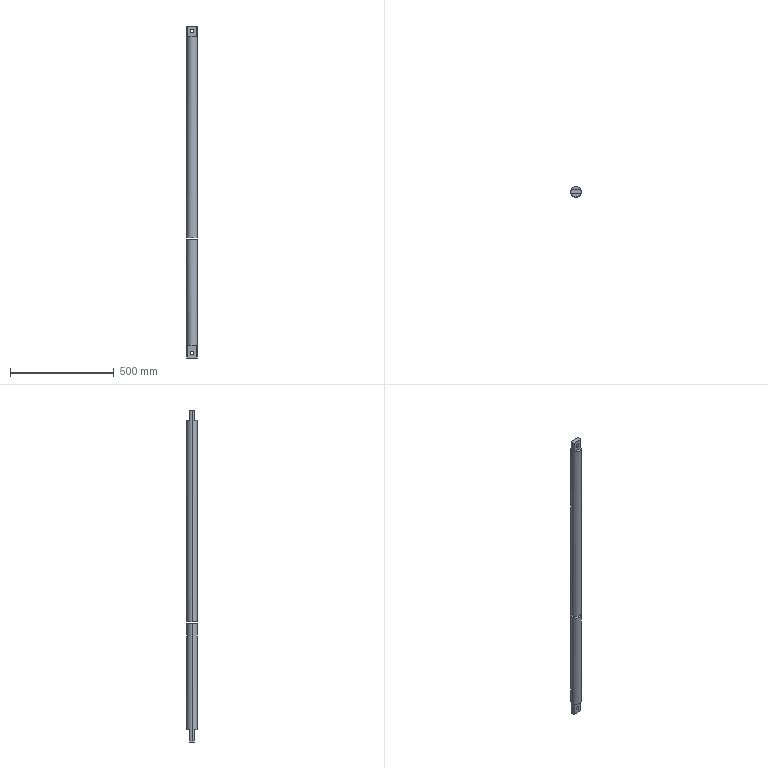Part | SolidWorks | features HoleWzd 2, ICE 2, MirrorPattern 2, Extrusion 1 | 2 solids | 20 faces | box 50 x 50 x 1600 mm | volume 3004412 mm3 | plane 12 | cylinder 8 | commonest cylinder face diameters 16.5 x4 50 x4
STEP:
#1=CARTESIAN_POINT('',(0.,10.,33.25));
#2=VERTEX_POINT('',#1);
#3=CARTESIAN_POINT('',(0.,10.,16.75));
#4=VERTEX_POINT('',#3);
#5=CARTESIAN_POINT('',(0.,10.,25.));
#6=DIRECTION('',(0.,-1.,0.));
#7=DIRECTION('',(0.,0.,-1.));
#8=AXIS2_PLACEMENT_3D('',#5,#6,#7);
#9=CIRCLE('',#8,8.25);
#10=EDGE_CURVE('',#2,#4,#9,.T.);
#11=ORIENTED_EDGE('',*,*,#10,.F.);
#12=CARTESIAN_POINT('',(0.,-10.,33.25));
#13=VERTEX_POINT('',#12);
#14=CARTESIAN_POINT('',(0.,-10.,33.25));
#15=DIRECTION('',(0.,-1.,0.));
#16=VECTOR('',#15,1000.);
#17=LINE('',#14,#16);
#18=EDGE_CURVE('',#2,#13,#17,.T.);
#19=ORIENTED_EDGE('',*,*,#18,.T.);
#20=CARTESIAN_POINT('',(0.,-10.,16.75));
#21=VERTEX_POINT('',#20);
#22=CARTESIAN_POINT('',(0.,-10.,25.));
#23=DIRECTION('',(0.,-1.,0.));
#24=DIRECTION('',(0.,0.,-1.));
#25=AXIS2_PLACEMENT_3D('',#22,#23,#24);
#26=CIRCLE('',#25,8.25);
#27=EDGE_CURVE('',#13,#21,#26,.T.);
#28=ORIENTED_EDGE('',*,*,#27,.T.);
#29=CARTESIAN_POINT('',(0.,-10.,16.75));
#30=DIRECTION('',(0.,-1.,0.));
#31=VECTOR('',#30,1000.);
#32=LINE('',#29,#31);
#33=EDGE_CURVE('',#4,#21,#32,.T.);
#34=ORIENTED_EDGE('',*,*,#33,.F.);
#35=EDGE_LOOP('',(#11,#19,#28,#34));
#36=FACE_OUTER_BOUND('',#35,.T.);
#37=CARTESIAN_POINT('',(0.,-10.,25.));
#38=DIRECTION('',(0.,-1.,0.));
#39=DIRECTION('',(0.,0.,-1.));
#40=AXIS2_PLACEMENT_3D('',#37,#38,#39);
#41=CYLINDRICAL_SURFACE('',#40,8.25);
#42=ADVANCED_FACE('',(#36),#41,.F.);
#43=CARTESIAN_POINT('',(25.,0.,569.));
#44=VERTEX_POINT('',#43);
#45=CARTESIAN_POINT('',(-25.,0.,569.));
#46=VERTEX_POINT('',#45);
#47=CARTESIAN_POINT('',(0.,0.,569.));
#48=DIRECTION('',(0.,0.,1.));
#49=DIRECTION('',(0.,-1.,0.));
#50=AXIS2_PLACEMENT_3D('',#47,#48,#49);
#51=CIRCLE('',#50,25.);
#52=EDGE_CURVE('',#44,#46,#51,.T.);
#53=ORIENTED_EDGE('',*,*,#52,.F.);
#54=CARTESIAN_POINT('',(25.,0.,0.));
#55=VERTEX_POINT('',#54);
#56=CARTESIAN_POINT('',(25.,0.,1600.));
#57=DIRECTION('',(0.,0.,-1.));
#58=VECTOR('',#57,1000.);
#59=LINE('',#56,#58);
#60=EDGE_CURVE('',#44,#55,#59,.T.);
#61=ORIENTED_EDGE('',*,*,#60,.T.);
#62=CARTESIAN_POINT('',(22.913,10.,0.));
#63=VERTEX_POINT('',#62);
#64=CARTESIAN_POINT('',(0.,0.,0.));
#65=DIRECTION('',(0.,0.,1.));
#66=DIRECTION('',(1.,0.,0.));
#67=AXIS2_PLACEMENT_3D('',#64,#65,#66);
#68=CIRCLE('',#67,25.);
#69=EDGE_CURVE('',#55,#63,#68,.T.);
#70=ORIENTED_EDGE('',*,*,#69,.T.);
#71=CARTESIAN_POINT('',(22.913,10.,60.));
#72=VERTEX_POINT('',#71);
#73=CARTESIAN_POINT('',(22.913,10.,1600.));
#74=DIRECTION('',(0.,0.,1.));
#75=VECTOR('',#74,1000.);
#76=LINE('',#73,#75);
#77=EDGE_CURVE('',#63,#72,#76,.T.);
#78=ORIENTED_EDGE('',*,*,#77,.T.);
#79=CARTESIAN_POINT('',(-22.913,10.,60.));
#80=VERTEX_POINT('',#79);
#81=CARTESIAN_POINT('',(0.,0.,60.));
#82=DIRECTION('',(0.,0.,-1.));
#83=DIRECTION('',(-1.,0.,0.));
#84=AXIS2_PLACEMENT_3D('',#81,#82,#83);
#85=CIRCLE('',#84,25.);
#86=EDGE_CURVE('',#80,#72,#85,.T.);
#87=ORIENTED_EDGE('',*,*,#86,.F.);
#88=CARTESIAN_POINT('',(-22.913,10.,0.));
#89=VERTEX_POINT('',#88);
#90=CARTESIAN_POINT('',(-22.913,10.,1600.));
#91=DIRECTION('',(0.,0.,-1.));
#92=VECTOR('',#91,1000.);
#93=LINE('',#90,#92);
#94=EDGE_CURVE('',#80,#89,#93,.T.);
#95=ORIENTED_EDGE('',*,*,#94,.T.);
#96=CARTESIAN_POINT('',(-25.,0.,0.));
#97=VERTEX_POINT('',#96);
#98=CARTESIAN_POINT('',(0.,0.,0.));
#99=DIRECTION('',(0.,0.,1.));
#100=DIRECTION('',(1.,0.,0.));
#101=AXIS2_PLACEMENT_3D('',#98,#99,#100);
#102=CIRCLE('',#101,25.);
#103=EDGE_CURVE('',#89,#97,#102,.T.);
#104=ORIENTED_EDGE('',*,*,#103,.T.);
#105=CARTESIAN_POINT('',(-25.,0.,1600.));
#106=DIRECTION('',(0.,0.,-1.));
#107=VECTOR('',#106,1000.);
#108=LINE('',#105,#107);
#109=EDGE_CURVE('',#46,#97,#108,.T.);
#110=ORIENTED_EDGE('',*,*,#109,.F.);
#111=EDGE_LOOP('',(#53,#61,#70,#78,#87,#95,#104,#110));
#112=FACE_OUTER_BOUND('',#111,.T.);
#113=CARTESIAN_POINT('',(0.,0.,1600.));
#114=DIRECTION('',(0.,0.,-1.));
#115=DIRECTION('',(-1.,0.,0.));
#116=AXIS2_PLACEMENT_3D('',#113,#114,#115);
#117=CYLINDRICAL_SURFACE('',#116,25.);
#118=ADVANCED_FACE('',(#112),#117,.T.);
#119=ORIENTED_EDGE('',*,*,#60,.F.);
#120=CARTESIAN_POINT('',(0.,0.,569.));
#121=DIRECTION('',(0.,0.,1.));
#122=DIRECTION('',(0.,-1.,0.));
#123=AXIS2_PLACEMENT_3D('',#120,#121,#122);
#124=CIRCLE('',#123,25.);
#125=EDGE_CURVE('',#46,#44,#124,.T.);
#126=ORIENTED_EDGE('',*,*,#125,.F.);
#127=ORIENTED_EDGE('',*,*,#109,.T.);
#128=CARTESIAN_POINT('',(-22.913,-10.,0.));
#129=VERTEX_POINT('',#128);
#130=CARTESIAN_POINT('',(0.,0.,0.));
#131=DIRECTION('',(0.,0.,1.));
#132=DIRECTION('',(1.,0.,0.));
#133=AXIS2_PLACEMENT_3D('',#130,#131,#132);
#134=CIRCLE('',#133,25.);
#135=EDGE_CURVE('',#97,#129,#134,.T.);
#136=ORIENTED_EDGE('',*,*,#135,.T.);
#137=CARTESIAN_POINT('',(-22.913,-10.,60.));
#138=VERTEX_POINT('',#137);
#139=CARTESIAN_POINT('',(-22.913,-10.,1600.));
#140=DIRECTION('',(0.,0.,1.));
#141=VECTOR('',#140,1000.);
#142=LINE('',#139,#141);
#143=EDGE_CURVE('',#129,#138,#142,.T.);
#144=ORIENTED_EDGE('',*,*,#143,.T.);
#145=CARTESIAN_POINT('',(22.913,-10.,60.));
#146=VERTEX_POINT('',#145);
#147=CARTESIAN_POINT('',(0.,0.,60.));
#148=DIRECTION('',(0.,0.,1.));
#149=DIRECTION('',(1.,0.,0.));
#150=AXIS2_PLACEMENT_3D('',#147,#148,#149);
#151=CIRCLE('',#150,25.);
#152=EDGE_CURVE('',#138,#146,#151,.T.);
#153=ORIENTED_EDGE('',*,*,#152,.T.);
#154=CARTESIAN_POINT('',(22.913,-10.,0.));
#155=VERTEX_POINT('',#154);
#156=CARTESIAN_POINT('',(22.913,-10.,1600.));
#157=DIRECTION('',(0.,0.,-1.));
#158=VECTOR('',#157,1000.);
#159=LINE('',#156,#158);
#160=EDGE_CURVE('',#146,#155,#159,.T.);
#161=ORIENTED_EDGE('',*,*,#160,.T.);
#162=CARTESIAN_POINT('',(0.,0.,0.));
#163=DIRECTION('',(0.,0.,1.));
#164=DIRECTION('',(1.,0.,0.));
#165=AXIS2_PLACEMENT_3D('',#162,#163,#164);
#166=CIRCLE('',#165,25.);
#167=EDGE_CURVE('',#155,#55,#166,.T.);
#168=ORIENTED_EDGE('',*,*,#167,.T.);
#169=EDGE_LOOP('',(#119,#126,#127,#136,#144,#153,#161,#168));
#170=FACE_OUTER_BOUND('',#169,.T.);
#171=CARTESIAN_POINT('',(0.,0.,1600.));
#172=DIRECTION('',(0.,0.,-1.));
#173=DIRECTION('',(-1.,0.,0.));
#174=AXIS2_PLACEMENT_3D('',#171,#172,#173);
#175=CYLINDRICAL_SURFACE('',#174,25.);
#176=ADVANCED_FACE('',(#170),#175,.T.);
#177=ORIENTED_EDGE('',*,*,#103,.F.);
#178=CARTESIAN_POINT('',(0.,10.,0.));
#179=DIRECTION('',(1.,0.,0.));
#180=VECTOR('',#179,1000.);
#181=LINE('',#178,#180);
#182=EDGE_CURVE('',#89,#63,#181,.T.);
#183=ORIENTED_EDGE('',*,*,#182,.T.);
#184=ORIENTED_EDGE('',*,*,#69,.F.);
#185=ORIENTED_EDGE('',*,*,#167,.F.);
#186=CARTESIAN_POINT('',(0.,-10.,0.));
#187=DIRECTION('',(-1.,0.,0.));
#188=VECTOR('',#187,1000.);
#189=LINE('',#186,#188);
#190=EDGE_CURVE('',#155,#129,#189,.T.);
#191=ORIENTED_EDGE('',*,*,#190,.T.);
#192=ORIENTED_EDGE('',*,*,#135,.F.);
#193=EDGE_LOOP('',(#177,#183,#184,#185,#191,#192));
#194=FACE_OUTER_BOUND('',#193,.T.);
#195=CARTESIAN_POINT('',(0.,0.,0.));
#196=DIRECTION('',(0.,0.,1.));
#197=DIRECTION('',(1.,0.,0.));
#198=AXIS2_PLACEMENT_3D('',#195,#196,#197);
#199=PLANE('',#198);
#200=ADVANCED_FACE('',(#194),#199,.F.);
#201=CARTESIAN_POINT('',(-25.,-10.,60.));
#202=DIRECTION('',(1.,0.,0.));
#203=VECTOR('',#202,1000.);
#204=LINE('',#201,#203);
#205=EDGE_CURVE('',#138,#146,#204,.T.);
#206=ORIENTED_EDGE('',*,*,#205,.T.);
#207=ORIENTED_EDGE('',*,*,#152,.F.);
#208=EDGE_LOOP('',(#206,#207));
#209=FACE_OUTER_BOUND('',#208,.T.);
#210=CARTESIAN_POINT('',(-25.,-1010.,60.));
#211=DIRECTION('',(0.,0.,1.));
#212=DIRECTION('',(1.,0.,0.));
#213=AXIS2_PLACEMENT_3D('',#210,#211,#212);
#214=PLANE('',#213);
#215=ADVANCED_FACE('',(#209),#214,.F.);
#216=CARTESIAN_POINT('',(0.,-10.,25.));
#217=DIRECTION('',(0.,-1.,0.));
#218=DIRECTION('',(0.,0.,-1.));
#219=AXIS2_PLACEMENT_3D('',#216,#217,#218);
#220=CIRCLE('',#219,8.25);
#221=EDGE_CURVE('',#21,#13,#220,.T.);
#222=ORIENTED_EDGE('',*,*,#221,.F.);
#223=ORIENTED_EDGE('',*,*,#27,.F.);
#224=EDGE_LOOP('',(#222,#223));
#225=FACE_BOUND('',#224,.T.);
#226=ORIENTED_EDGE('',*,*,#205,.F.);
#227=ORIENTED_EDGE('',*,*,#143,.F.);
#228=ORIENTED_EDGE('',*,*,#190,.F.);
#229=ORIENTED_EDGE('',*,*,#160,.F.);
#230=EDGE_LOOP('',(#226,#227,#228,#229));
#231=FACE_OUTER_BOUND('',#230,.T.);
#232=CARTESIAN_POINT('',(0.,-10.,0.));
#233=DIRECTION('',(0.,1.,0.));
#234=DIRECTION('',(0.,0.,1.));
#235=AXIS2_PLACEMENT_3D('',#232,#233,#234);
#236=PLANE('',#235);
#237=ADVANCED_FACE('',(#225,#231),#236,.F.);
#238=ORIENTED_EDGE('',*,*,#86,.T.);
#239=CARTESIAN_POINT('',(-25.,10.,60.));
#240=DIRECTION('',(1.,0.,0.));
#241=VECTOR('',#240,1000.);
#242=LINE('',#239,#241);
#243=EDGE_CURVE('',#80,#72,#242,.T.);
#244=ORIENTED_EDGE('',*,*,#243,.F.);
#245=EDGE_LOOP('',(#238,#244));
#246=FACE_OUTER_BOUND('',#245,.T.);
#247=CARTESIAN_POINT('',(-25.,1010.,60.));
#248=DIRECTION('',(0.,0.,-1.));
#249=DIRECTION('',(-1.,0.,0.));
#250=AXIS2_PLACEMENT_3D('',#247,#248,#249);
#251=PLANE('',#250);
#252=ADVANCED_FACE('',(#246),#251,.T.);
#253=CARTESIAN_POINT('',(0.,10.,25.));
#254=DIRECTION('',(0.,-1.,0.));
#255=DIRECTION('',(0.,0.,-1.));
#256=AXIS2_PLACEMENT_3D('',#253,#254,#255);
#257=CIRCLE('',#256,8.25);
#258=EDGE_CURVE('',#4,#2,#257,.T.);
#259=ORIENTED_EDGE('',*,*,#258,.T.);
#260=ORIENTED_EDGE('',*,*,#10,.T.);
#261=EDGE_LOOP('',(#259,#260));
#262=FACE_BOUND('',#261,.T.);
#263=ORIENTED_EDGE('',*,*,#243,.T.);
#264=ORIENTED_EDGE('',*,*,#77,.F.);
#265=ORIENTED_EDGE('',*,*,#182,.F.);
#266=ORIENTED_EDGE('',*,*,#94,.F.);
#267=EDGE_LOOP('',(#263,#264,#265,#266));
#268=FACE_OUTER_BOUND('',#267,.T.);
#269=CARTESIAN_POINT('',(0.,10.,0.));
#270=DIRECTION('',(0.,-1.,0.));
#271=DIRECTION('',(0.,0.,1.));
#272=AXIS2_PLACEMENT_3D('',#269,#270,#271);
#273=PLANE('',#272);
#274=ADVANCED_FACE('',(#262,#268),#273,.F.);
#275=ORIENTED_EDGE('',*,*,#18,.F.);
#276=ORIENTED_EDGE('',*,*,#258,.F.);
#277=ORIENTED_EDGE('',*,*,#33,.T.);
#278=ORIENTED_EDGE('',*,*,#221,.T.);
#279=EDGE_LOOP('',(#275,#276,#277,#278));
#280=FACE_OUTER_BOUND('',#279,.T.);
#281=CARTESIAN_POINT('',(0.,-10.,25.));
#282=DIRECTION('',(0.,-1.,0.));
#283=DIRECTION('',(0.,0.,-1.));
#284=AXIS2_PLACEMENT_3D('',#281,#282,#283);
#285=CYLINDRICAL_SURFACE('',#284,8.25);
#286=ADVANCED_FACE('',(#280),#285,.F.);
#287=ORIENTED_EDGE('',*,*,#125,.T.);
#288=ORIENTED_EDGE('',*,*,#52,.T.);
#289=EDGE_LOOP('',(#287,#288));
#290=FACE_OUTER_BOUND('',#289,.T.);
#291=CARTESIAN_POINT('',(0.,0.,569.));
#292=DIRECTION('',(0.,0.,1.));
#293=DIRECTION('',(0.,1.,0.));
#294=AXIS2_PLACEMENT_3D('',#291,#292,#293);
#295=PLANE('',#294);
#296=ADVANCED_FACE('',(#290),#295,.T.);
#297=CLOSED_SHELL('',(#42,#118,#176,#200,#215,#237,#252,#274,#286,#296));
#298=MANIFOLD_SOLID_BREP('',#297);
#299=CARTESIAN_POINT('',(25.,0.,1600.));
#300=VERTEX_POINT('',#299);
#301=CARTESIAN_POINT('',(22.913,10.,1600.));
#302=VERTEX_POINT('',#301);
#303=CARTESIAN_POINT('',(0.,0.,1600.));
#304=DIRECTION('',(0.,0.,1.));
#305=DIRECTION('',(1.,0.,0.));
#306=AXIS2_PLACEMENT_3D('',#303,#304,#305);
#307=CIRCLE('',#306,25.);
#308=EDGE_CURVE('',#300,#302,#307,.T.);
#309=ORIENTED_EDGE('',*,*,#308,.F.);
#310=CARTESIAN_POINT('',(25.,0.,579.));
#311=VERTEX_POINT('',#310);
#312=CARTESIAN_POINT('',(25.,0.,1600.));
#313=DIRECTION('',(0.,0.,-1.));
#314=VECTOR('',#313,1000.);
#315=LINE('',#312,#314);
#316=EDGE_CURVE('',#300,#311,#315,.T.);
#317=ORIENTED_EDGE('',*,*,#316,.T.);
#318=CARTESIAN_POINT('',(-25.,0.,579.));
#319=VERTEX_POINT('',#318);
#320=CARTESIAN_POINT('',(0.,0.,579.));
#321=DIRECTION('',(0.,0.,1.));
#322=DIRECTION('',(0.,-1.,0.));
#323=AXIS2_PLACEMENT_3D('',#320,#321,#322);
#324=CIRCLE('',#323,25.);
#325=EDGE_CURVE('',#311,#319,#324,.T.);
#326=ORIENTED_EDGE('',*,*,#325,.T.);
#327=CARTESIAN_POINT('',(-25.,0.,1600.));
#328=VERTEX_POINT('',#327);
#329=CARTESIAN_POINT('',(-25.,0.,1600.));
#330=DIRECTION('',(0.,0.,-1.));
#331=VECTOR('',#330,1000.);
#332=LINE('',#329,#331);
#333=EDGE_CURVE('',#328,#319,#332,.T.);
#334=ORIENTED_EDGE('',*,*,#333,.F.);
#335=CARTESIAN_POINT('',(-22.913,10.,1600.));
#336=VERTEX_POINT('',#335);
#337=CARTESIAN_POINT('',(0.,0.,1600.));
#338=DIRECTION('',(0.,0.,1.));
#339=DIRECTION('',(1.,0.,0.));
#340=AXIS2_PLACEMENT_3D('',#337,#338,#339);
#341=CIRCLE('',#340,25.);
#342=EDGE_CURVE('',#336,#328,#341,.T.);
#343=ORIENTED_EDGE('',*,*,#342,.F.);
#344=CARTESIAN_POINT('',(-22.913,10.,1550.));
#345=VERTEX_POINT('',#344);
#346=CARTESIAN_POINT('',(-22.913,10.,1600.));
#347=DIRECTION('',(0.,0.,1.));
#348=VECTOR('',#347,1000.);
#349=LINE('',#346,#348);
#350=EDGE_CURVE('',#345,#336,#349,.T.);
#351=ORIENTED_EDGE('',*,*,#350,.F.);
#352=CARTESIAN_POINT('',(22.913,10.,1550.));
#353=VERTEX_POINT('',#352);
#354=CARTESIAN_POINT('',(0.,0.,1550.));
#355=DIRECTION('',(0.,0.,1.));
#356=DIRECTION('',(1.,0.,0.));
#357=AXIS2_PLACEMENT_3D('',#354,#355,#356);
#358=CIRCLE('',#357,25.);
#359=EDGE_CURVE('',#353,#345,#358,.T.);
#360=ORIENTED_EDGE('',*,*,#359,.F.);
#361=CARTESIAN_POINT('',(22.913,10.,1600.));
#362=DIRECTION('',(0.,0.,-1.));
#363=VECTOR('',#362,1000.);
#364=LINE('',#361,#363);
#365=EDGE_CURVE('',#302,#353,#364,.T.);
#366=ORIENTED_EDGE('',*,*,#365,.F.);
#367=EDGE_LOOP('',(#309,#317,#326,#334,#343,#351,#360,#366));
#368=FACE_OUTER_BOUND('',#367,.T.);
#369=CARTESIAN_POINT('',(0.,0.,1600.));
#370=DIRECTION('',(0.,0.,-1.));
#371=DIRECTION('',(-1.,0.,0.));
#372=AXIS2_PLACEMENT_3D('',#369,#370,#371);
#373=CYLINDRICAL_SURFACE('',#372,25.);
#374=ADVANCED_FACE('',(#368),#373,.T.);
#375=CARTESIAN_POINT('',(0.,10.,1566.75));
#376=VERTEX_POINT('',#375);
#377=CARTESIAN_POINT('',(0.,10.,1583.25));
#378=VERTEX_POINT('',#377);
#379=CARTESIAN_POINT('',(0.,10.,1575.));
#380=DIRECTION('',(0.,1.,0.));
#381=DIRECTION('',(0.,0.,1.));
#382=AXIS2_PLACEMENT_3D('',#379,#380,#381);
#383=CIRCLE('',#382,8.25);
#384=EDGE_CURVE('',#376,#378,#383,.T.);
#385=ORIENTED_EDGE('',*,*,#384,.T.);
#386=CARTESIAN_POINT('',(0.,-10.,1583.25));
#387=VERTEX_POINT('',#386);
#388=CARTESIAN_POINT('',(0.,-10.,1583.25));
#389=DIRECTION('',(0.,-1.,0.));
#390=VECTOR('',#389,1000.);
#391=LINE('',#388,#390);
#392=EDGE_CURVE('',#378,#387,#391,.T.);
#393=ORIENTED_EDGE('',*,*,#392,.T.);
#394=CARTESIAN_POINT('',(0.,-10.,1566.75));
#395=VERTEX_POINT('',#394);
#396=CARTESIAN_POINT('',(0.,-10.,1575.));
#397=DIRECTION('',(0.,-1.,0.));
#398=DIRECTION('',(0.,0.,-1.));
#399=AXIS2_PLACEMENT_3D('',#396,#397,#398);
#400=CIRCLE('',#399,8.25);
#401=EDGE_CURVE('',#387,#395,#400,.T.);
#402=ORIENTED_EDGE('',*,*,#401,.T.);
#403=CARTESIAN_POINT('',(0.,-10.,1566.75));
#404=DIRECTION('',(0.,-1.,0.));
#405=VECTOR('',#404,1000.);
#406=LINE('',#403,#405);
#407=EDGE_CURVE('',#376,#395,#406,.T.);
#408=ORIENTED_EDGE('',*,*,#407,.F.);
#409=EDGE_LOOP('',(#385,#393,#402,#408));
#410=FACE_OUTER_BOUND('',#409,.T.);
#411=CARTESIAN_POINT('',(0.,-10.,1575.));
#412=DIRECTION('',(0.,-1.,0.));
#413=DIRECTION('',(0.,0.,-1.));
#414=AXIS2_PLACEMENT_3D('',#411,#412,#413);
#415=CYLINDRICAL_SURFACE('',#414,8.25);
#416=ADVANCED_FACE('',(#410),#415,.F.);
#417=ORIENTED_EDGE('',*,*,#392,.F.);
#418=CARTESIAN_POINT('',(0.,10.,1575.));
#419=DIRECTION('',(0.,1.,0.));
#420=DIRECTION('',(0.,0.,1.));
#421=AXIS2_PLACEMENT_3D('',#418,#419,#420);
#422=CIRCLE('',#421,8.25);
#423=EDGE_CURVE('',#378,#376,#422,.T.);
#424=ORIENTED_EDGE('',*,*,#423,.T.);
#425=ORIENTED_EDGE('',*,*,#407,.T.);
#426=CARTESIAN_POINT('',(0.,-10.,1575.));
#427=DIRECTION('',(0.,-1.,0.));
#428=DIRECTION('',(0.,0.,-1.));
#429=AXIS2_PLACEMENT_3D('',#426,#427,#428);
#430=CIRCLE('',#429,8.25);
#431=EDGE_CURVE('',#395,#387,#430,.T.);
#432=ORIENTED_EDGE('',*,*,#431,.T.);
#433=EDGE_LOOP('',(#417,#424,#425,#432));
#434=FACE_OUTER_BOUND('',#433,.T.);
#435=CARTESIAN_POINT('',(0.,-10.,1575.));
#436=DIRECTION('',(0.,-1.,0.));
#437=DIRECTION('',(0.,0.,-1.));
#438=AXIS2_PLACEMENT_3D('',#435,#436,#437);
#439=CYLINDRICAL_SURFACE('',#438,8.25);
#440=ADVANCED_FACE('',(#434),#439,.F.);
#441=CARTESIAN_POINT('',(22.913,-10.,1550.));
#442=VERTEX_POINT('',#441);
#443=CARTESIAN_POINT('',(-22.913,-10.,1550.));
#444=VERTEX_POINT('',#443);
#445=CARTESIAN_POINT('',(25.,-10.,1550.));
#446=DIRECTION('',(-1.,0.,0.));
#447=VECTOR('',#446,1000.);
#448=LINE('',#445,#447);
#449=EDGE_CURVE('',#442,#444,#448,.T.);
#450=ORIENTED_EDGE('',*,*,#449,.T.);
#451=CARTESIAN_POINT('',(0.,0.,1550.));
#452=DIRECTION('',(0.,0.,-1.));
#453=DIRECTION('',(-1.,0.,0.));
#454=AXIS2_PLACEMENT_3D('',#451,#452,#453);
#455=CIRCLE('',#454,25.);
#456=EDGE_CURVE('',#442,#444,#455,.T.);
#457=ORIENTED_EDGE('',*,*,#456,.F.);
#458=EDGE_LOOP('',(#450,#457));
#459=FACE_OUTER_BOUND('',#458,.T.);
#460=CARTESIAN_POINT('',(25.,-1010.,1550.));
#461=DIRECTION('',(0.,0.,-1.));
#462=DIRECTION('',(-1.,0.,0.));
#463=AXIS2_PLACEMENT_3D('',#460,#461,#462);
#464=PLANE('',#463);
#465=ADVANCED_FACE('',(#459),#464,.F.);
#466=ORIENTED_EDGE('',*,*,#359,.T.);
#467=CARTESIAN_POINT('',(25.,10.,1550.));
#468=DIRECTION('',(-1.,0.,0.));
#469=VECTOR('',#468,1000.);
#470=LINE('',#467,#469);
#471=EDGE_CURVE('',#353,#345,#470,.T.);
#472=ORIENTED_EDGE('',*,*,#471,.F.);
#473=EDGE_LOOP('',(#466,#472));
#474=FACE_OUTER_BOUND('',#473,.T.);
#475=CARTESIAN_POINT('',(25.,1010.,1550.));
#476=DIRECTION('',(0.,0.,1.));
#477=DIRECTION('',(1.,0.,0.));
#478=AXIS2_PLACEMENT_3D('',#475,#476,#477);
#479=PLANE('',#478);
#480=ADVANCED_FACE('',(#474),#479,.T.);
#481=ORIENTED_EDGE('',*,*,#384,.F.);
#482=ORIENTED_EDGE('',*,*,#423,.F.);
#483=EDGE_LOOP('',(#481,#482));
#484=FACE_BOUND('',#483,.T.);
#485=ORIENTED_EDGE('',*,*,#365,.T.);
#486=ORIENTED_EDGE('',*,*,#471,.T.);
#487=ORIENTED_EDGE('',*,*,#350,.T.);
#488=CARTESIAN_POINT('',(0.,10.,1600.));
#489=DIRECTION('',(-1.,0.,0.));
#490=VECTOR('',#489,1000.);
#491=LINE('',#488,#490);
#492=EDGE_CURVE('',#302,#336,#491,.T.);
#493=ORIENTED_EDGE('',*,*,#492,.F.);
#494=EDGE_LOOP('',(#485,#486,#487,#493));
#495=FACE_OUTER_BOUND('',#494,.T.);
#496=CARTESIAN_POINT('',(0.,10.,0.));
#497=DIRECTION('',(0.,1.,0.));
#498=DIRECTION('',(0.,0.,1.));
#499=AXIS2_PLACEMENT_3D('',#496,#497,#498);
#500=PLANE('',#499);
#501=ADVANCED_FACE('',(#484,#495),#500,.T.);
#502=ORIENTED_EDGE('',*,*,#342,.T.);
#503=CARTESIAN_POINT('',(-22.913,-10.,1600.));
#504=VERTEX_POINT('',#503);
#505=CARTESIAN_POINT('',(0.,0.,1600.));
#506=DIRECTION('',(0.,0.,1.));
#507=DIRECTION('',(1.,0.,0.));
#508=AXIS2_PLACEMENT_3D('',#505,#506,#507);
#509=CIRCLE('',#508,25.);
#510=EDGE_CURVE('',#328,#504,#509,.T.);
#511=ORIENTED_EDGE('',*,*,#510,.T.);
#512=CARTESIAN_POINT('',(22.913,-10.,1600.));
#513=VERTEX_POINT('',#512);
#514=CARTESIAN_POINT('',(0.,-10.,1600.));
#515=DIRECTION('',(1.,0.,0.));
#516=VECTOR('',#515,1000.);
#517=LINE('',#514,#516);
#518=EDGE_CURVE('',#504,#513,#517,.T.);
#519=ORIENTED_EDGE('',*,*,#518,.T.);
#520=CARTESIAN_POINT('',(0.,0.,1600.));
#521=DIRECTION('',(0.,0.,1.));
#522=DIRECTION('',(1.,0.,0.));
#523=AXIS2_PLACEMENT_3D('',#520,#521,#522);
#524=CIRCLE('',#523,25.);
#525=EDGE_CURVE('',#513,#300,#524,.T.);
#526=ORIENTED_EDGE('',*,*,#525,.T.);
#527=ORIENTED_EDGE('',*,*,#308,.T.);
#528=ORIENTED_EDGE('',*,*,#492,.T.);
#529=EDGE_LOOP('',(#502,#511,#519,#526,#527,#528));
#530=FACE_OUTER_BOUND('',#529,.T.);
#531=CARTESIAN_POINT('',(0.,0.,1600.));
#532=DIRECTION('',(0.,0.,1.));
#533=DIRECTION('',(1.,0.,0.));
#534=AXIS2_PLACEMENT_3D('',#531,#532,#533);
#535=PLANE('',#534);
#536=ADVANCED_FACE('',(#530),#535,.T.);
#537=ORIENTED_EDGE('',*,*,#431,.F.);
#538=ORIENTED_EDGE('',*,*,#401,.F.);
#539=EDGE_LOOP('',(#537,#538));
#540=FACE_BOUND('',#539,.T.);
#541=CARTESIAN_POINT('',(-22.913,-10.,1600.));
#542=DIRECTION('',(0.,0.,-1.));
#543=VECTOR('',#542,1000.);
#544=LINE('',#541,#543);
#545=EDGE_CURVE('',#504,#444,#544,.T.);
#546=ORIENTED_EDGE('',*,*,#545,.T.);
#547=ORIENTED_EDGE('',*,*,#449,.F.);
#548=CARTESIAN_POINT('',(22.913,-10.,1600.));
#549=DIRECTION('',(0.,0.,1.));
#550=VECTOR('',#549,1000.);
#551=LINE('',#548,#550);
#552=EDGE_CURVE('',#442,#513,#551,.T.);
#553=ORIENTED_EDGE('',*,*,#552,.T.);
#554=ORIENTED_EDGE('',*,*,#518,.F.);
#555=EDGE_LOOP('',(#546,#547,#553,#554));
#556=FACE_OUTER_BOUND('',#555,.T.);
#557=CARTESIAN_POINT('',(0.,-10.,0.));
#558=DIRECTION('',(0.,-1.,0.));
#559=DIRECTION('',(0.,0.,1.));
#560=AXIS2_PLACEMENT_3D('',#557,#558,#559);
#561=PLANE('',#560);
#562=ADVANCED_FACE('',(#540,#556),#561,.T.);
#563=ORIENTED_EDGE('',*,*,#316,.F.);
#564=ORIENTED_EDGE('',*,*,#525,.F.);
#565=ORIENTED_EDGE('',*,*,#552,.F.);
#566=ORIENTED_EDGE('',*,*,#456,.T.);
#567=ORIENTED_EDGE('',*,*,#545,.F.);
#568=ORIENTED_EDGE('',*,*,#510,.F.);
#569=ORIENTED_EDGE('',*,*,#333,.T.);
#570=CARTESIAN_POINT('',(0.,0.,579.));
#571=DIRECTION('',(0.,0.,1.));
#572=DIRECTION('',(0.,-1.,0.));
#573=AXIS2_PLACEMENT_3D('',#570,#571,#572);
#574=CIRCLE('',#573,25.);
#575=EDGE_CURVE('',#319,#311,#574,.T.);
#576=ORIENTED_EDGE('',*,*,#575,.T.);
#577=EDGE_LOOP('',(#563,#564,#565,#566,#567,#568,#569,#576));
#578=FACE_OUTER_BOUND('',#577,.T.);
#579=CARTESIAN_POINT('',(0.,0.,1600.));
#580=DIRECTION('',(0.,0.,-1.));
#581=DIRECTION('',(-1.,0.,0.));
#582=AXIS2_PLACEMENT_3D('',#579,#580,#581);
#583=CYLINDRICAL_SURFACE('',#582,25.);
#584=ADVANCED_FACE('',(#578),#583,.T.);
#585=ORIENTED_EDGE('',*,*,#575,.F.);
#586=ORIENTED_EDGE('',*,*,#325,.F.);
#587=EDGE_LOOP('',(#585,#586));
#588=FACE_OUTER_BOUND('',#587,.T.);
#589=CARTESIAN_POINT('',(0.,0.,579.));
#590=DIRECTION('',(0.,0.,1.));
#591=DIRECTION('',(0.,1.,0.));
#592=AXIS2_PLACEMENT_3D('',#589,#590,#591);
#593=PLANE('',#592);
#594=ADVANCED_FACE('',(#588),#593,.F.);
#595=CLOSED_SHELL('',(#374,#416,#440,#465,#480,#501,#536,#562,#584,#594));
#596=MANIFOLD_SOLID_BREP('',#595);
#597=CARTESIAN_POINT('',(0.,0.,0.));
#598=DIRECTION('',(0.,0.,1.));
#599=DIRECTION('',(1.,0.,0.));
#600=AXIS2_PLACEMENT_3D('',#597,#598,#599);
#601=(LENGTH_UNIT()NAMED_UNIT(*)SI_UNIT(.MILLI.,.METRE.));
#602=UNCERTAINTY_MEASURE_WITH_UNIT(LENGTH_MEASURE(0.00001),#601,'','');
#603=(NAMED_UNIT(*)PLANE_ANGLE_UNIT()SI_UNIT($,.RADIAN.));
#604=(NAMED_UNIT(*)SI_UNIT($,.STERADIAN.)SOLID_ANGLE_UNIT());
#605=(GEOMETRIC_REPRESENTATION_CONTEXT(3)GLOBAL_UNCERTAINTY_ASSIGNED_CONTEXT((#602))GLOBAL_UNIT_ASSIGNED_CONTEXT((#601,#603,#604))REPRESENTATION_CONTEXT('',''));
#606=ADVANCED_BREP_SHAPE_REPRESENTATION('',(#298,#596,#600),#605);